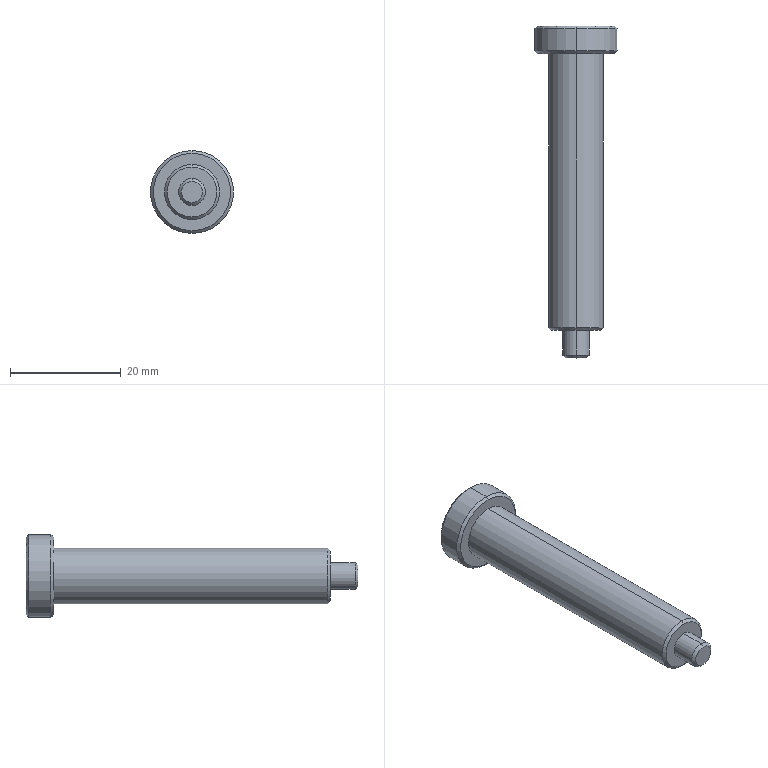Part | SolidWorks | features Chamfer 1, Revolution 1 | 1 solid | 18 faces | box 15 x 60 x 15 mm | volume 4886 mm3 | cone 8 | cylinder 6 | plane 4 | commonest cylinder face diameters 4.85 x2 10 x2 15 x2
STEP:
#1=CARTESIAN_POINT('',(0.,-60.,-1.925));
#2=VERTEX_POINT('',#1);
#3=CARTESIAN_POINT('',(0.,-60.,1.925));
#4=VERTEX_POINT('',#3);
#5=CARTESIAN_POINT('',(0.,-60.,0.));
#6=DIRECTION('',(0.,-1.,0.));
#7=DIRECTION('',(0.,0.,1.));
#8=AXIS2_PLACEMENT_3D('',#5,#6,#7);
#9=CIRCLE('',#8,1.925);
#10=EDGE_CURVE('',#2,#4,#9,.T.);
#11=ORIENTED_EDGE('',*,*,#10,.F.);
#12=CARTESIAN_POINT('',(0.,-59.5,-2.425));
#13=VERTEX_POINT('',#12);
#14=CARTESIAN_POINT('',(0.,-59.5,-2.425));
#15=DIRECTION('',(0.,0.7071,-0.7071));
#16=VECTOR('',#15,1000.);
#17=LINE('',#14,#16);
#18=EDGE_CURVE('',#2,#13,#17,.T.);
#19=ORIENTED_EDGE('',*,*,#18,.T.);
#20=CARTESIAN_POINT('',(0.,-59.5,2.425));
#21=VERTEX_POINT('',#20);
#22=CARTESIAN_POINT('',(0.,-59.5,0.));
#23=DIRECTION('',(0.,1.,0.));
#24=DIRECTION('',(0.,0.,1.));
#25=AXIS2_PLACEMENT_3D('',#22,#23,#24);
#26=CIRCLE('',#25,2.425);
#27=EDGE_CURVE('',#21,#13,#26,.T.);
#28=ORIENTED_EDGE('',*,*,#27,.F.);
#29=CARTESIAN_POINT('',(0.,-59.5,2.425));
#30=DIRECTION('',(0.,0.7071,0.7071));
#31=VECTOR('',#30,1000.);
#32=LINE('',#29,#31);
#33=EDGE_CURVE('',#4,#21,#32,.T.);
#34=ORIENTED_EDGE('',*,*,#33,.F.);
#35=EDGE_LOOP('',(#11,#19,#28,#34));
#36=FACE_OUTER_BOUND('',#35,.T.);
#37=CARTESIAN_POINT('',(0.,-59.5,0.));
#38=DIRECTION('',(0.,1.,0.));
#39=DIRECTION('',(0.,0.,1.));
#40=AXIS2_PLACEMENT_3D('',#37,#38,#39);
#41=CONICAL_SURFACE('',#40,2.425,0.7854);
#42=ADVANCED_FACE('',(#36),#41,.T.);
#43=CARTESIAN_POINT('',(0.,-55.,-4.5));
#44=VERTEX_POINT('',#43);
#45=CARTESIAN_POINT('',(0.,-55.,4.5));
#46=VERTEX_POINT('',#45);
#47=CARTESIAN_POINT('',(0.,-55.,0.));
#48=DIRECTION('',(0.,-1.,0.));
#49=DIRECTION('',(0.,0.,1.));
#50=AXIS2_PLACEMENT_3D('',#47,#48,#49);
#51=CIRCLE('',#50,4.5);
#52=EDGE_CURVE('',#44,#46,#51,.T.);
#53=ORIENTED_EDGE('',*,*,#52,.F.);
#54=CARTESIAN_POINT('',(0.,-54.5,-5.));
#55=VERTEX_POINT('',#54);
#56=CARTESIAN_POINT('',(0.,-54.5,-5.));
#57=DIRECTION('',(0.,0.7071,-0.7071));
#58=VECTOR('',#57,1000.);
#59=LINE('',#56,#58);
#60=EDGE_CURVE('',#44,#55,#59,.T.);
#61=ORIENTED_EDGE('',*,*,#60,.T.);
#62=CARTESIAN_POINT('',(0.,-54.5,5.));
#63=VERTEX_POINT('',#62);
#64=CARTESIAN_POINT('',(0.,-54.5,0.));
#65=DIRECTION('',(0.,1.,0.));
#66=DIRECTION('',(0.,0.,1.));
#67=AXIS2_PLACEMENT_3D('',#64,#65,#66);
#68=CIRCLE('',#67,5.);
#69=EDGE_CURVE('',#63,#55,#68,.T.);
#70=ORIENTED_EDGE('',*,*,#69,.F.);
#71=CARTESIAN_POINT('',(0.,-54.5,5.));
#72=DIRECTION('',(0.,0.7071,0.7071));
#73=VECTOR('',#72,1000.);
#74=LINE('',#71,#73);
#75=EDGE_CURVE('',#46,#63,#74,.T.);
#76=ORIENTED_EDGE('',*,*,#75,.F.);
#77=EDGE_LOOP('',(#53,#61,#70,#76));
#78=FACE_OUTER_BOUND('',#77,.T.);
#79=CARTESIAN_POINT('',(0.,-54.5,0.));
#80=DIRECTION('',(0.,1.,0.));
#81=DIRECTION('',(0.,0.,1.));
#82=AXIS2_PLACEMENT_3D('',#79,#80,#81);
#83=CONICAL_SURFACE('',#82,5.,0.7854);
#84=ADVANCED_FACE('',(#78),#83,.T.);
#85=CARTESIAN_POINT('',(0.,-5.,-7.));
#86=VERTEX_POINT('',#85);
#87=CARTESIAN_POINT('',(0.,-5.,7.));
#88=VERTEX_POINT('',#87);
#89=CARTESIAN_POINT('',(0.,-5.,0.));
#90=DIRECTION('',(0.,-1.,0.));
#91=DIRECTION('',(0.,0.,1.));
#92=AXIS2_PLACEMENT_3D('',#89,#90,#91);
#93=CIRCLE('',#92,7.);
#94=EDGE_CURVE('',#86,#88,#93,.T.);
#95=ORIENTED_EDGE('',*,*,#94,.F.);
#96=CARTESIAN_POINT('',(0.,-4.5,-7.5));
#97=VERTEX_POINT('',#96);
#98=CARTESIAN_POINT('',(0.,-4.5,-7.5));
#99=DIRECTION('',(0.,0.7071,-0.7071));
#100=VECTOR('',#99,1000.);
#101=LINE('',#98,#100);
#102=EDGE_CURVE('',#86,#97,#101,.T.);
#103=ORIENTED_EDGE('',*,*,#102,.T.);
#104=CARTESIAN_POINT('',(0.,-4.5,7.5));
#105=VERTEX_POINT('',#104);
#106=CARTESIAN_POINT('',(0.,-4.5,0.));
#107=DIRECTION('',(0.,1.,0.));
#108=DIRECTION('',(0.,0.,1.));
#109=AXIS2_PLACEMENT_3D('',#106,#107,#108);
#110=CIRCLE('',#109,7.5);
#111=EDGE_CURVE('',#105,#97,#110,.T.);
#112=ORIENTED_EDGE('',*,*,#111,.F.);
#113=CARTESIAN_POINT('',(0.,-4.5,7.5));
#114=DIRECTION('',(0.,0.7071,0.7071));
#115=VECTOR('',#114,1000.);
#116=LINE('',#113,#115);
#117=EDGE_CURVE('',#88,#105,#116,.T.);
#118=ORIENTED_EDGE('',*,*,#117,.F.);
#119=EDGE_LOOP('',(#95,#103,#112,#118));
#120=FACE_OUTER_BOUND('',#119,.T.);
#121=CARTESIAN_POINT('',(0.,-4.5,0.));
#122=DIRECTION('',(0.,1.,0.));
#123=DIRECTION('',(0.,0.,1.));
#124=AXIS2_PLACEMENT_3D('',#121,#122,#123);
#125=CONICAL_SURFACE('',#124,7.5,0.7854);
#126=ADVANCED_FACE('',(#120),#125,.T.);
#127=CARTESIAN_POINT('',(0.,0.,7.));
#128=VERTEX_POINT('',#127);
#129=CARTESIAN_POINT('',(0.,0.,-7.));
#130=VERTEX_POINT('',#129);
#131=CARTESIAN_POINT('',(0.,0.,0.));
#132=DIRECTION('',(0.,1.,0.));
#133=DIRECTION('',(0.,0.,-1.));
#134=AXIS2_PLACEMENT_3D('',#131,#132,#133);
#135=CIRCLE('',#134,7.);
#136=EDGE_CURVE('',#128,#130,#135,.T.);
#137=ORIENTED_EDGE('',*,*,#136,.F.);
#138=CARTESIAN_POINT('',(0.,-0.5,7.5));
#139=VERTEX_POINT('',#138);
#140=CARTESIAN_POINT('',(0.,0.,7.));
#141=DIRECTION('',(0.,-0.7071,0.7071));
#142=VECTOR('',#141,1000.);
#143=LINE('',#140,#142);
#144=EDGE_CURVE('',#128,#139,#143,.T.);
#145=ORIENTED_EDGE('',*,*,#144,.T.);
#146=CARTESIAN_POINT('',(0.,-0.5,-7.5));
#147=VERTEX_POINT('',#146);
#148=CARTESIAN_POINT('',(0.,-0.5,0.));
#149=DIRECTION('',(0.,-1.,0.));
#150=DIRECTION('',(0.,0.,-1.));
#151=AXIS2_PLACEMENT_3D('',#148,#149,#150);
#152=CIRCLE('',#151,7.5);
#153=EDGE_CURVE('',#147,#139,#152,.T.);
#154=ORIENTED_EDGE('',*,*,#153,.F.);
#155=CARTESIAN_POINT('',(0.,0.,-7.));
#156=DIRECTION('',(0.,-0.7071,-0.7071));
#157=VECTOR('',#156,1000.);
#158=LINE('',#155,#157);
#159=EDGE_CURVE('',#130,#147,#158,.T.);
#160=ORIENTED_EDGE('',*,*,#159,.F.);
#161=EDGE_LOOP('',(#137,#145,#154,#160));
#162=FACE_OUTER_BOUND('',#161,.T.);
#163=CARTESIAN_POINT('',(0.,0.,0.));
#164=DIRECTION('',(0.,-1.,0.));
#165=DIRECTION('',(0.,0.,-1.));
#166=AXIS2_PLACEMENT_3D('',#163,#164,#165);
#167=CONICAL_SURFACE('',#166,7.,0.7854);
#168=ADVANCED_FACE('',(#162),#167,.T.);
#169=ORIENTED_EDGE('',*,*,#27,.T.);
#170=CARTESIAN_POINT('',(0.,-55.,-2.425));
#171=VERTEX_POINT('',#170);
#172=CARTESIAN_POINT('',(0.,0.,-2.425));
#173=DIRECTION('',(0.,1.,0.));
#174=VECTOR('',#173,1000.);
#175=LINE('',#172,#174);
#176=EDGE_CURVE('',#13,#171,#175,.T.);
#177=ORIENTED_EDGE('',*,*,#176,.T.);
#178=CARTESIAN_POINT('',(0.,-55.,2.425));
#179=VERTEX_POINT('',#178);
#180=CARTESIAN_POINT('',(0.,-55.,0.));
#181=DIRECTION('',(0.,1.,0.));
#182=DIRECTION('',(0.,0.,1.));
#183=AXIS2_PLACEMENT_3D('',#180,#181,#182);
#184=CIRCLE('',#183,2.425);
#185=EDGE_CURVE('',#179,#171,#184,.T.);
#186=ORIENTED_EDGE('',*,*,#185,.F.);
#187=CARTESIAN_POINT('',(0.,0.,2.425));
#188=DIRECTION('',(0.,1.,0.));
#189=VECTOR('',#188,1000.);
#190=LINE('',#187,#189);
#191=EDGE_CURVE('',#21,#179,#190,.T.);
#192=ORIENTED_EDGE('',*,*,#191,.F.);
#193=EDGE_LOOP('',(#169,#177,#186,#192));
#194=FACE_OUTER_BOUND('',#193,.T.);
#195=CARTESIAN_POINT('',(0.,0.,0.));
#196=DIRECTION('',(0.,1.,0.));
#197=DIRECTION('',(0.,0.,1.));
#198=AXIS2_PLACEMENT_3D('',#195,#196,#197);
#199=CYLINDRICAL_SURFACE('',#198,2.425);
#200=ADVANCED_FACE('',(#194),#199,.T.);
#201=ORIENTED_EDGE('',*,*,#69,.T.);
#202=CARTESIAN_POINT('',(0.,-5.,-5.));
#203=VERTEX_POINT('',#202);
#204=CARTESIAN_POINT('',(0.,0.,-5.));
#205=DIRECTION('',(0.,1.,0.));
#206=VECTOR('',#205,1000.);
#207=LINE('',#204,#206);
#208=EDGE_CURVE('',#55,#203,#207,.T.);
#209=ORIENTED_EDGE('',*,*,#208,.T.);
#210=CARTESIAN_POINT('',(0.,-5.,5.));
#211=VERTEX_POINT('',#210);
#212=CARTESIAN_POINT('',(0.,-5.,0.));
#213=DIRECTION('',(0.,1.,0.));
#214=DIRECTION('',(0.,0.,1.));
#215=AXIS2_PLACEMENT_3D('',#212,#213,#214);
#216=CIRCLE('',#215,5.);
#217=EDGE_CURVE('',#211,#203,#216,.T.);
#218=ORIENTED_EDGE('',*,*,#217,.F.);
#219=CARTESIAN_POINT('',(0.,0.,5.));
#220=DIRECTION('',(0.,1.,0.));
#221=VECTOR('',#220,1000.);
#222=LINE('',#219,#221);
#223=EDGE_CURVE('',#63,#211,#222,.T.);
#224=ORIENTED_EDGE('',*,*,#223,.F.);
#225=EDGE_LOOP('',(#201,#209,#218,#224));
#226=FACE_OUTER_BOUND('',#225,.T.);
#227=CARTESIAN_POINT('',(0.,0.,0.));
#228=DIRECTION('',(0.,1.,0.));
#229=DIRECTION('',(0.,0.,1.));
#230=AXIS2_PLACEMENT_3D('',#227,#228,#229);
#231=CYLINDRICAL_SURFACE('',#230,5.);
#232=ADVANCED_FACE('',(#226),#231,.T.);
#233=ORIENTED_EDGE('',*,*,#111,.T.);
#234=CARTESIAN_POINT('',(0.,0.,-7.5));
#235=DIRECTION('',(0.,1.,0.));
#236=VECTOR('',#235,1000.);
#237=LINE('',#234,#236);
#238=EDGE_CURVE('',#97,#147,#237,.T.);
#239=ORIENTED_EDGE('',*,*,#238,.T.);
#240=ORIENTED_EDGE('',*,*,#153,.T.);
#241=CARTESIAN_POINT('',(0.,0.,7.5));
#242=DIRECTION('',(0.,1.,0.));
#243=VECTOR('',#242,1000.);
#244=LINE('',#241,#243);
#245=EDGE_CURVE('',#105,#139,#244,.T.);
#246=ORIENTED_EDGE('',*,*,#245,.F.);
#247=EDGE_LOOP('',(#233,#239,#240,#246));
#248=FACE_OUTER_BOUND('',#247,.T.);
#249=CARTESIAN_POINT('',(0.,0.,0.));
#250=DIRECTION('',(0.,1.,0.));
#251=DIRECTION('',(0.,0.,1.));
#252=AXIS2_PLACEMENT_3D('',#249,#250,#251);
#253=CYLINDRICAL_SURFACE('',#252,7.5);
#254=ADVANCED_FACE('',(#248),#253,.T.);
#255=CARTESIAN_POINT('',(0.,0.,0.));
#256=DIRECTION('',(0.,1.,0.));
#257=DIRECTION('',(0.,0.,-1.));
#258=AXIS2_PLACEMENT_3D('',#255,#256,#257);
#259=CIRCLE('',#258,7.);
#260=EDGE_CURVE('',#130,#128,#259,.T.);
#261=ORIENTED_EDGE('',*,*,#260,.T.);
#262=ORIENTED_EDGE('',*,*,#136,.T.);
#263=EDGE_LOOP('',(#261,#262));
#264=FACE_OUTER_BOUND('',#263,.T.);
#265=CARTESIAN_POINT('',(0.,0.,0.));
#266=DIRECTION('',(0.,-1.,0.));
#267=DIRECTION('',(0.,0.,-1.));
#268=AXIS2_PLACEMENT_3D('',#265,#266,#267);
#269=PLANE('',#268);
#270=ADVANCED_FACE('',(#264),#269,.F.);
#271=ORIENTED_EDGE('',*,*,#238,.F.);
#272=CARTESIAN_POINT('',(0.,-4.5,0.));
#273=DIRECTION('',(0.,1.,0.));
#274=DIRECTION('',(0.,0.,1.));
#275=AXIS2_PLACEMENT_3D('',#272,#273,#274);
#276=CIRCLE('',#275,7.5);
#277=EDGE_CURVE('',#97,#105,#276,.T.);
#278=ORIENTED_EDGE('',*,*,#277,.T.);
#279=ORIENTED_EDGE('',*,*,#245,.T.);
#280=CARTESIAN_POINT('',(0.,-0.5,0.));
#281=DIRECTION('',(0.,-1.,0.));
#282=DIRECTION('',(0.,0.,-1.));
#283=AXIS2_PLACEMENT_3D('',#280,#281,#282);
#284=CIRCLE('',#283,7.5);
#285=EDGE_CURVE('',#139,#147,#284,.T.);
#286=ORIENTED_EDGE('',*,*,#285,.T.);
#287=EDGE_LOOP('',(#271,#278,#279,#286));
#288=FACE_OUTER_BOUND('',#287,.T.);
#289=CARTESIAN_POINT('',(0.,0.,0.));
#290=DIRECTION('',(0.,1.,0.));
#291=DIRECTION('',(0.,0.,1.));
#292=AXIS2_PLACEMENT_3D('',#289,#290,#291);
#293=CYLINDRICAL_SURFACE('',#292,7.5);
#294=ADVANCED_FACE('',(#288),#293,.T.);
#295=CARTESIAN_POINT('',(0.,-5.,0.));
#296=DIRECTION('',(0.,-1.,0.));
#297=DIRECTION('',(0.,0.,1.));
#298=AXIS2_PLACEMENT_3D('',#295,#296,#297);
#299=CIRCLE('',#298,7.);
#300=EDGE_CURVE('',#88,#86,#299,.T.);
#301=ORIENTED_EDGE('',*,*,#300,.T.);
#302=ORIENTED_EDGE('',*,*,#94,.T.);
#303=EDGE_LOOP('',(#301,#302));
#304=FACE_OUTER_BOUND('',#303,.T.);
#305=ORIENTED_EDGE('',*,*,#217,.T.);
#306=CARTESIAN_POINT('',(0.,-5.,0.));
#307=DIRECTION('',(0.,1.,0.));
#308=DIRECTION('',(0.,0.,1.));
#309=AXIS2_PLACEMENT_3D('',#306,#307,#308);
#310=CIRCLE('',#309,5.);
#311=EDGE_CURVE('',#203,#211,#310,.T.);
#312=ORIENTED_EDGE('',*,*,#311,.T.);
#313=EDGE_LOOP('',(#305,#312));
#314=FACE_BOUND('',#313,.T.);
#315=CARTESIAN_POINT('',(0.,-5.,-7.5));
#316=DIRECTION('',(0.,1.,0.));
#317=DIRECTION('',(0.,0.,1.));
#318=AXIS2_PLACEMENT_3D('',#315,#316,#317);
#319=PLANE('',#318);
#320=ADVANCED_FACE('',(#304,#314),#319,.F.);
#321=ORIENTED_EDGE('',*,*,#208,.F.);
#322=CARTESIAN_POINT('',(0.,-54.5,0.));
#323=DIRECTION('',(0.,1.,0.));
#324=DIRECTION('',(0.,0.,1.));
#325=AXIS2_PLACEMENT_3D('',#322,#323,#324);
#326=CIRCLE('',#325,5.);
#327=EDGE_CURVE('',#55,#63,#326,.T.);
#328=ORIENTED_EDGE('',*,*,#327,.T.);
#329=ORIENTED_EDGE('',*,*,#223,.T.);
#330=ORIENTED_EDGE('',*,*,#311,.F.);
#331=EDGE_LOOP('',(#321,#328,#329,#330));
#332=FACE_OUTER_BOUND('',#331,.T.);
#333=CARTESIAN_POINT('',(0.,0.,0.));
#334=DIRECTION('',(0.,1.,0.));
#335=DIRECTION('',(0.,0.,1.));
#336=AXIS2_PLACEMENT_3D('',#333,#334,#335);
#337=CYLINDRICAL_SURFACE('',#336,5.);
#338=ADVANCED_FACE('',(#332),#337,.T.);
#339=CARTESIAN_POINT('',(0.,-55.,0.));
#340=DIRECTION('',(0.,-1.,0.));
#341=DIRECTION('',(0.,0.,1.));
#342=AXIS2_PLACEMENT_3D('',#339,#340,#341);
#343=CIRCLE('',#342,4.5);
#344=EDGE_CURVE('',#46,#44,#343,.T.);
#345=ORIENTED_EDGE('',*,*,#344,.T.);
#346=ORIENTED_EDGE('',*,*,#52,.T.);
#347=EDGE_LOOP('',(#345,#346));
#348=FACE_OUTER_BOUND('',#347,.T.);
#349=ORIENTED_EDGE('',*,*,#185,.T.);
#350=CARTESIAN_POINT('',(0.,-55.,0.));
#351=DIRECTION('',(0.,1.,0.));
#352=DIRECTION('',(0.,0.,1.));
#353=AXIS2_PLACEMENT_3D('',#350,#351,#352);
#354=CIRCLE('',#353,2.425);
#355=EDGE_CURVE('',#171,#179,#354,.T.);
#356=ORIENTED_EDGE('',*,*,#355,.T.);
#357=EDGE_LOOP('',(#349,#356));
#358=FACE_BOUND('',#357,.T.);
#359=CARTESIAN_POINT('',(0.,-55.,-5.));
#360=DIRECTION('',(0.,1.,0.));
#361=DIRECTION('',(0.,0.,1.));
#362=AXIS2_PLACEMENT_3D('',#359,#360,#361);
#363=PLANE('',#362);
#364=ADVANCED_FACE('',(#348,#358),#363,.F.);
#365=ORIENTED_EDGE('',*,*,#176,.F.);
#366=CARTESIAN_POINT('',(0.,-59.5,0.));
#367=DIRECTION('',(0.,1.,0.));
#368=DIRECTION('',(0.,0.,1.));
#369=AXIS2_PLACEMENT_3D('',#366,#367,#368);
#370=CIRCLE('',#369,2.425);
#371=EDGE_CURVE('',#13,#21,#370,.T.);
#372=ORIENTED_EDGE('',*,*,#371,.T.);
#373=ORIENTED_EDGE('',*,*,#191,.T.);
#374=ORIENTED_EDGE('',*,*,#355,.F.);
#375=EDGE_LOOP('',(#365,#372,#373,#374));
#376=FACE_OUTER_BOUND('',#375,.T.);
#377=CARTESIAN_POINT('',(0.,0.,0.));
#378=DIRECTION('',(0.,1.,0.));
#379=DIRECTION('',(0.,0.,1.));
#380=AXIS2_PLACEMENT_3D('',#377,#378,#379);
#381=CYLINDRICAL_SURFACE('',#380,2.425);
#382=ADVANCED_FACE('',(#376),#381,.T.);
#383=CARTESIAN_POINT('',(0.,-60.,0.));
#384=DIRECTION('',(0.,-1.,0.));
#385=DIRECTION('',(0.,0.,1.));
#386=AXIS2_PLACEMENT_3D('',#383,#384,#385);
#387=CIRCLE('',#386,1.925);
#388=EDGE_CURVE('',#4,#2,#387,.T.);
#389=ORIENTED_EDGE('',*,*,#388,.T.);
#390=ORIENTED_EDGE('',*,*,#10,.T.);
#391=EDGE_LOOP('',(#389,#390));
#392=FACE_OUTER_BOUND('',#391,.T.);
#393=CARTESIAN_POINT('',(0.,-60.,-2.425));
#394=DIRECTION('',(0.,1.,0.));
#395=DIRECTION('',(0.,0.,1.));
#396=AXIS2_PLACEMENT_3D('',#393,#394,#395);
#397=PLANE('',#396);
#398=ADVANCED_FACE('',(#392),#397,.F.);
#399=ORIENTED_EDGE('',*,*,#144,.F.);
#400=ORIENTED_EDGE('',*,*,#260,.F.);
#401=ORIENTED_EDGE('',*,*,#159,.T.);
#402=ORIENTED_EDGE('',*,*,#285,.F.);
#403=EDGE_LOOP('',(#399,#400,#401,#402));
#404=FACE_OUTER_BOUND('',#403,.T.);
#405=CARTESIAN_POINT('',(0.,0.,0.));
#406=DIRECTION('',(0.,-1.,0.));
#407=DIRECTION('',(0.,0.,-1.));
#408=AXIS2_PLACEMENT_3D('',#405,#406,#407);
#409=CONICAL_SURFACE('',#408,7.,0.7854);
#410=ADVANCED_FACE('',(#404),#409,.T.);
#411=ORIENTED_EDGE('',*,*,#102,.F.);
#412=ORIENTED_EDGE('',*,*,#300,.F.);
#413=ORIENTED_EDGE('',*,*,#117,.T.);
#414=ORIENTED_EDGE('',*,*,#277,.F.);
#415=EDGE_LOOP('',(#411,#412,#413,#414));
#416=FACE_OUTER_BOUND('',#415,.T.);
#417=CARTESIAN_POINT('',(0.,-4.5,0.));
#418=DIRECTION('',(0.,1.,0.));
#419=DIRECTION('',(0.,0.,1.));
#420=AXIS2_PLACEMENT_3D('',#417,#418,#419);
#421=CONICAL_SURFACE('',#420,7.5,0.7854);
#422=ADVANCED_FACE('',(#416),#421,.T.);
#423=ORIENTED_EDGE('',*,*,#60,.F.);
#424=ORIENTED_EDGE('',*,*,#344,.F.);
#425=ORIENTED_EDGE('',*,*,#75,.T.);
#426=ORIENTED_EDGE('',*,*,#327,.F.);
#427=EDGE_LOOP('',(#423,#424,#425,#426));
#428=FACE_OUTER_BOUND('',#427,.T.);
#429=CARTESIAN_POINT('',(0.,-54.5,0.));
#430=DIRECTION('',(0.,1.,0.));
#431=DIRECTION('',(0.,0.,1.));
#432=AXIS2_PLACEMENT_3D('',#429,#430,#431);
#433=CONICAL_SURFACE('',#432,5.,0.7854);
#434=ADVANCED_FACE('',(#428),#433,.T.);
#435=ORIENTED_EDGE('',*,*,#18,.F.);
#436=ORIENTED_EDGE('',*,*,#388,.F.);
#437=ORIENTED_EDGE('',*,*,#33,.T.);
#438=ORIENTED_EDGE('',*,*,#371,.F.);
#439=EDGE_LOOP('',(#435,#436,#437,#438));
#440=FACE_OUTER_BOUND('',#439,.T.);
#441=CARTESIAN_POINT('',(0.,-59.5,0.));
#442=DIRECTION('',(0.,1.,0.));
#443=DIRECTION('',(0.,0.,1.));
#444=AXIS2_PLACEMENT_3D('',#441,#442,#443);
#445=CONICAL_SURFACE('',#444,2.425,0.7854);
#446=ADVANCED_FACE('',(#440),#445,.T.);
#447=CLOSED_SHELL('',(#42,#84,#126,#168,#200,#232,#254,#270,#294,#320,#338,#364,#382,#398,#410,#422,#434,#446));
#448=MANIFOLD_SOLID_BREP('',#447);
#449=CARTESIAN_POINT('',(0.,0.,0.));
#450=DIRECTION('',(0.,0.,1.));
#451=DIRECTION('',(1.,0.,0.));
#452=AXIS2_PLACEMENT_3D('',#449,#450,#451);
#453=(LENGTH_UNIT()NAMED_UNIT(*)SI_UNIT(.MILLI.,.METRE.));
#454=UNCERTAINTY_MEASURE_WITH_UNIT(LENGTH_MEASURE(0.00001),#453,'','');
#455=(NAMED_UNIT(*)PLANE_ANGLE_UNIT()SI_UNIT($,.RADIAN.));
#456=(NAMED_UNIT(*)SI_UNIT($,.STERADIAN.)SOLID_ANGLE_UNIT());
#457=(GEOMETRIC_REPRESENTATION_CONTEXT(3)GLOBAL_UNCERTAINTY_ASSIGNED_CONTEXT((#454))GLOBAL_UNIT_ASSIGNED_CONTEXT((#453,#455,#456))REPRESENTATION_CONTEXT('',''));
#458=ADVANCED_BREP_SHAPE_REPRESENTATION('',(#448,#452),#457);